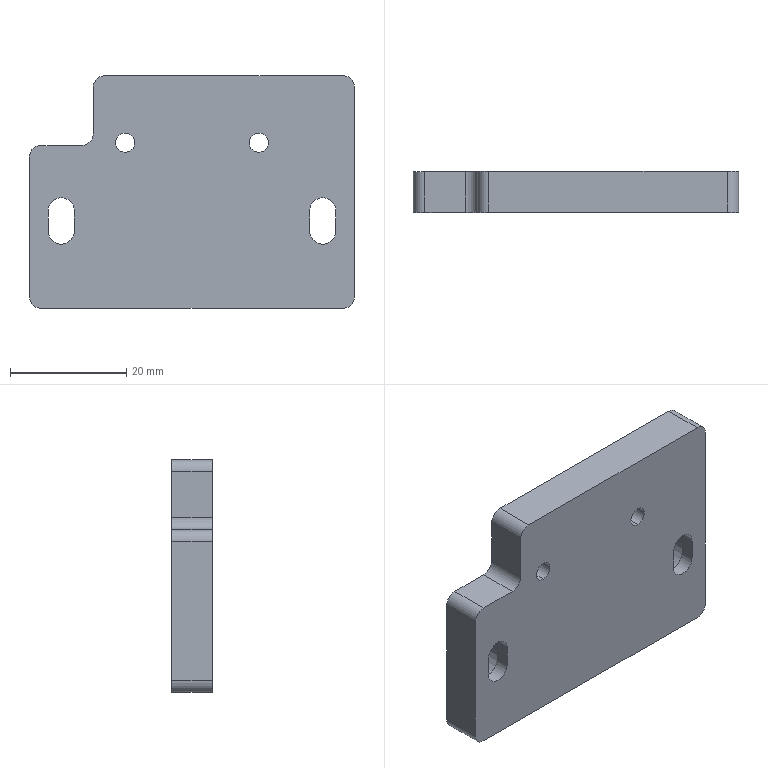Part | STEP file | 1 solid | 40 faces | box 56 x 7 x 40 mm | volume 13740 mm3 | cylinder 22 | plane 18 | commonest cylinder face diameters 4 x6 4.5 x6 8 x6 3.3 x4